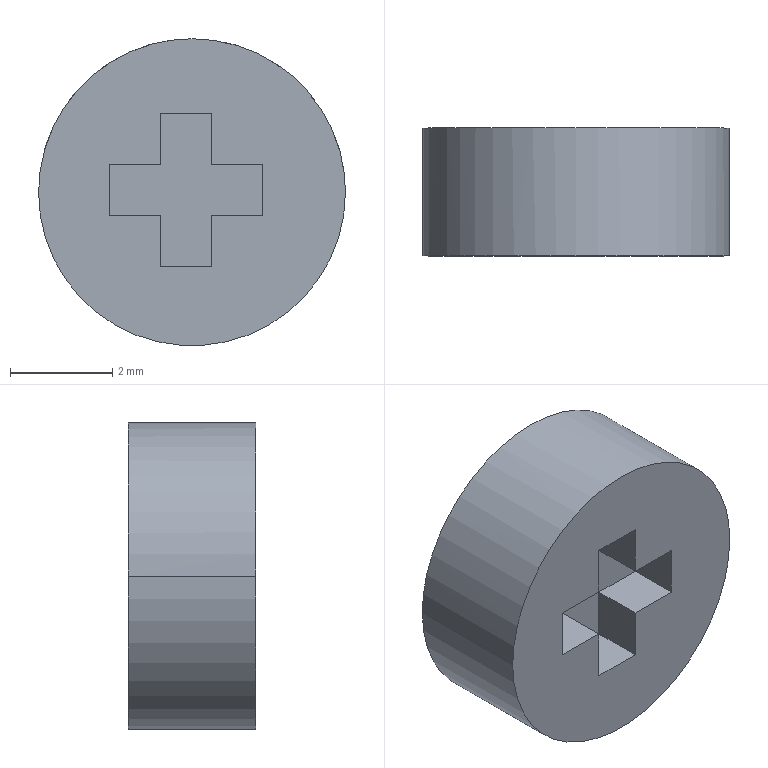Part | STEP file | Positioning_id1914_x_t | 1 solid | 17 faces | box 6 x 2.5 x 6 mm | volume 65.686 mm3 | plane 15 | cylinder 2 | commonest cylinder face diameters 6 x2
STEP:
#1=CARTESIAN_POINT('',(0.,0.,0.));
#2=DIRECTION('',(0.,0.,1.));
#3=DIRECTION('',(1.,0.,0.));
#4=AXIS2_PLACEMENT_3D('',#1,#2,#3);
#5=CARTESIAN_POINT('',(-766.532,-35.,479.288));
#6=VERTEX_POINT('',#5);
#7=CARTESIAN_POINT('',(-766.532,-35.,478.288));
#8=VERTEX_POINT('',#7);
#9=CARTESIAN_POINT('',(-766.532,-35.,479.288));
#10=DIRECTION('',(0.,0.,-1.));
#11=VECTOR('',#10,1.);
#12=LINE('',#9,#11);
#13=CARTESIAN_POINT('',(-766.532,-35.,478.288));
#14=DIRECTION('',(0.,1.,0.));
#15=DIRECTION('',(1.,0.,0.));
#16=AXIS2_PLACEMENT_3D('',#13,#14,#15);
#17=PLANE('',#16);
#18=CARTESIAN_POINT('',(0.,-1.));
#19=DIRECTION('',(0.,1.));
#20=VECTOR('',#19,1.);
#21=LINE('',#18,#20);
#22=(GEOMETRIC_REPRESENTATION_CONTEXT(2)PARAMETRIC_REPRESENTATION_CONTEXT()REPRESENTATION_CONTEXT('',''));
#23=DEFINITIONAL_REPRESENTATION('',(#21),#22);
#24=PCURVE('',#17,#23);
#25=CARTESIAN_POINT('',(-766.532,-35.,478.288));
#26=DIRECTION('',(-1.,0.,0.));
#27=DIRECTION('',(0.,0.,1.));
#28=AXIS2_PLACEMENT_3D('',#25,#26,#27);
#29=PLANE('',#28);
#30=CARTESIAN_POINT('',(1.,0.));
#31=DIRECTION('',(-1.,0.));
#32=VECTOR('',#31,1.);
#33=LINE('',#30,#32);
#34=(GEOMETRIC_REPRESENTATION_CONTEXT(2)PARAMETRIC_REPRESENTATION_CONTEXT()REPRESENTATION_CONTEXT('',''));
#35=DEFINITIONAL_REPRESENTATION('',(#33),#34);
#36=PCURVE('',#29,#35);
#37=SURFACE_CURVE('',#12,(#24,#36),.PCURVE_S1.);
#38=EDGE_CURVE('',#6,#8,#37,.T.);
#39=ORIENTED_EDGE('',*,*,#38,.F.);
#40=CARTESIAN_POINT('',(-767.532,-35.,479.288));
#41=VERTEX_POINT('',#40);
#42=CARTESIAN_POINT('',(-767.532,-35.,479.288));
#43=DIRECTION('',(1.,0.,0.));
#44=VECTOR('',#43,1.);
#45=LINE('',#42,#44);
#46=CARTESIAN_POINT('',(-1.,-1.));
#47=DIRECTION('',(1.,0.));
#48=VECTOR('',#47,1.);
#49=LINE('',#46,#48);
#50=(GEOMETRIC_REPRESENTATION_CONTEXT(2)PARAMETRIC_REPRESENTATION_CONTEXT()REPRESENTATION_CONTEXT('',''));
#51=DEFINITIONAL_REPRESENTATION('',(#49),#50);
#52=PCURVE('',#17,#51);
#53=CARTESIAN_POINT('',(-766.532,-35.,479.288));
#54=DIRECTION('',(0.,0.,-1.));
#55=DIRECTION('',(-1.,0.,0.));
#56=AXIS2_PLACEMENT_3D('',#53,#54,#55);
#57=PLANE('',#56);
#58=CARTESIAN_POINT('',(1.,0.));
#59=DIRECTION('',(-1.,0.));
#60=VECTOR('',#59,1.);
#61=LINE('',#58,#60);
#62=(GEOMETRIC_REPRESENTATION_CONTEXT(2)PARAMETRIC_REPRESENTATION_CONTEXT()REPRESENTATION_CONTEXT('',''));
#63=DEFINITIONAL_REPRESENTATION('',(#61),#62);
#64=PCURVE('',#57,#63);
#65=SURFACE_CURVE('',#45,(#52,#64),.PCURVE_S1.);
#66=EDGE_CURVE('',#41,#6,#65,.T.);
#67=ORIENTED_EDGE('',*,*,#66,.F.);
#68=CARTESIAN_POINT('',(-767.532,-35.,480.288));
#69=VERTEX_POINT('',#68);
#70=CARTESIAN_POINT('',(-767.532,-35.,480.288));
#71=DIRECTION('',(0.,0.,-1.));
#72=VECTOR('',#71,1.);
#73=LINE('',#70,#72);
#74=CARTESIAN_POINT('',(-1.,-2.));
#75=DIRECTION('',(0.,1.));
#76=VECTOR('',#75,1.);
#77=LINE('',#74,#76);
#78=(GEOMETRIC_REPRESENTATION_CONTEXT(2)PARAMETRIC_REPRESENTATION_CONTEXT()REPRESENTATION_CONTEXT('',''));
#79=DEFINITIONAL_REPRESENTATION('',(#77),#78);
#80=PCURVE('',#17,#79);
#81=CARTESIAN_POINT('',(-767.532,-35.,480.288));
#82=DIRECTION('',(-1.,0.,0.));
#83=DIRECTION('',(0.,0.,1.));
#84=AXIS2_PLACEMENT_3D('',#81,#82,#83);
#85=PLANE('',#84);
#86=CARTESIAN_POINT('',(0.,0.));
#87=DIRECTION('',(-1.,0.));
#88=VECTOR('',#87,1.);
#89=LINE('',#86,#88);
#90=(GEOMETRIC_REPRESENTATION_CONTEXT(2)PARAMETRIC_REPRESENTATION_CONTEXT()REPRESENTATION_CONTEXT('',''));
#91=DEFINITIONAL_REPRESENTATION('',(#89),#90);
#92=PCURVE('',#85,#91);
#93=SURFACE_CURVE('',#73,(#80,#92),.PCURVE_S1.);
#94=EDGE_CURVE('',#69,#41,#93,.T.);
#95=ORIENTED_EDGE('',*,*,#94,.F.);
#96=CARTESIAN_POINT('',(-768.532,-35.,480.288));
#97=VERTEX_POINT('',#96);
#98=CARTESIAN_POINT('',(-768.532,-35.,480.288));
#99=DIRECTION('',(1.,0.,0.));
#100=VECTOR('',#99,1.);
#101=LINE('',#98,#100);
#102=CARTESIAN_POINT('',(-2.,-2.));
#103=DIRECTION('',(1.,0.));
#104=VECTOR('',#103,1.);
#105=LINE('',#102,#104);
#106=(GEOMETRIC_REPRESENTATION_CONTEXT(2)PARAMETRIC_REPRESENTATION_CONTEXT()REPRESENTATION_CONTEXT('',''));
#107=DEFINITIONAL_REPRESENTATION('',(#105),#106);
#108=PCURVE('',#17,#107);
#109=CARTESIAN_POINT('',(-768.532,-35.,480.288));
#110=DIRECTION('',(0.,0.,-1.));
#111=DIRECTION('',(-1.,0.,0.));
#112=AXIS2_PLACEMENT_3D('',#109,#110,#111);
#113=PLANE('',#112);
#114=CARTESIAN_POINT('',(0.,0.));
#115=DIRECTION('',(-1.,0.));
#116=VECTOR('',#115,1.);
#117=LINE('',#114,#116);
#118=(GEOMETRIC_REPRESENTATION_CONTEXT(2)PARAMETRIC_REPRESENTATION_CONTEXT()REPRESENTATION_CONTEXT('',''));
#119=DEFINITIONAL_REPRESENTATION('',(#117),#118);
#120=PCURVE('',#113,#119);
#121=SURFACE_CURVE('',#101,(#108,#120),.PCURVE_S1.);
#122=EDGE_CURVE('',#97,#69,#121,.T.);
#123=ORIENTED_EDGE('',*,*,#122,.F.);
#124=CARTESIAN_POINT('',(-768.532,-35.,479.288));
#125=VERTEX_POINT('',#124);
#126=CARTESIAN_POINT('',(-768.532,-35.,479.288));
#127=DIRECTION('',(0.,0.,1.));
#128=VECTOR('',#127,1.);
#129=LINE('',#126,#128);
#130=CARTESIAN_POINT('',(-2.,-1.));
#131=DIRECTION('',(0.,-1.));
#132=VECTOR('',#131,1.);
#133=LINE('',#130,#132);
#134=(GEOMETRIC_REPRESENTATION_CONTEXT(2)PARAMETRIC_REPRESENTATION_CONTEXT()REPRESENTATION_CONTEXT('',''));
#135=DEFINITIONAL_REPRESENTATION('',(#133),#134);
#136=PCURVE('',#17,#135);
#137=CARTESIAN_POINT('',(-768.532,-35.,479.288));
#138=DIRECTION('',(1.,0.,0.));
#139=DIRECTION('',(0.,0.,-1.));
#140=AXIS2_PLACEMENT_3D('',#137,#138,#139);
#141=PLANE('',#140);
#142=CARTESIAN_POINT('',(0.,0.));
#143=DIRECTION('',(-1.,0.));
#144=VECTOR('',#143,1.);
#145=LINE('',#142,#144);
#146=(GEOMETRIC_REPRESENTATION_CONTEXT(2)PARAMETRIC_REPRESENTATION_CONTEXT()REPRESENTATION_CONTEXT('',''));
#147=DEFINITIONAL_REPRESENTATION('',(#145),#146);
#148=PCURVE('',#141,#147);
#149=SURFACE_CURVE('',#129,(#136,#148),.PCURVE_S1.);
#150=EDGE_CURVE('',#125,#97,#149,.T.);
#151=ORIENTED_EDGE('',*,*,#150,.F.);
#152=CARTESIAN_POINT('',(-769.532,-35.,479.288));
#153=VERTEX_POINT('',#152);
#154=CARTESIAN_POINT('',(-769.532,-35.,479.288));
#155=DIRECTION('',(1.,0.,0.));
#156=VECTOR('',#155,1.);
#157=LINE('',#154,#156);
#158=CARTESIAN_POINT('',(-3.,-1.));
#159=DIRECTION('',(1.,0.));
#160=VECTOR('',#159,1.);
#161=LINE('',#158,#160);
#162=(GEOMETRIC_REPRESENTATION_CONTEXT(2)PARAMETRIC_REPRESENTATION_CONTEXT()REPRESENTATION_CONTEXT('',''));
#163=DEFINITIONAL_REPRESENTATION('',(#161),#162);
#164=PCURVE('',#17,#163);
#165=CARTESIAN_POINT('',(-768.532,-35.,479.288));
#166=DIRECTION('',(0.,0.,-1.));
#167=DIRECTION('',(-1.,0.,0.));
#168=AXIS2_PLACEMENT_3D('',#165,#166,#167);
#169=PLANE('',#168);
#170=CARTESIAN_POINT('',(1.,0.));
#171=DIRECTION('',(-1.,0.));
#172=VECTOR('',#171,1.);
#173=LINE('',#170,#172);
#174=(GEOMETRIC_REPRESENTATION_CONTEXT(2)PARAMETRIC_REPRESENTATION_CONTEXT()REPRESENTATION_CONTEXT('',''));
#175=DEFINITIONAL_REPRESENTATION('',(#173),#174);
#176=PCURVE('',#169,#175);
#177=SURFACE_CURVE('',#157,(#164,#176),.PCURVE_S1.);
#178=EDGE_CURVE('',#153,#125,#177,.T.);
#179=ORIENTED_EDGE('',*,*,#178,.F.);
#180=CARTESIAN_POINT('',(-769.532,-35.,478.288));
#181=VERTEX_POINT('',#180);
#182=CARTESIAN_POINT('',(-769.532,-35.,478.288));
#183=DIRECTION('',(0.,0.,1.));
#184=VECTOR('',#183,1.);
#185=LINE('',#182,#184);
#186=CARTESIAN_POINT('',(-3.,0.));
#187=DIRECTION('',(0.,-1.));
#188=VECTOR('',#187,1.);
#189=LINE('',#186,#188);
#190=(GEOMETRIC_REPRESENTATION_CONTEXT(2)PARAMETRIC_REPRESENTATION_CONTEXT()REPRESENTATION_CONTEXT('',''));
#191=DEFINITIONAL_REPRESENTATION('',(#189),#190);
#192=PCURVE('',#17,#191);
#193=CARTESIAN_POINT('',(-769.532,-35.,479.288));
#194=DIRECTION('',(1.,0.,0.));
#195=DIRECTION('',(0.,0.,-1.));
#196=AXIS2_PLACEMENT_3D('',#193,#194,#195);
#197=PLANE('',#196);
#198=CARTESIAN_POINT('',(1.,0.));
#199=DIRECTION('',(-1.,0.));
#200=VECTOR('',#199,1.);
#201=LINE('',#198,#200);
#202=(GEOMETRIC_REPRESENTATION_CONTEXT(2)PARAMETRIC_REPRESENTATION_CONTEXT()REPRESENTATION_CONTEXT('',''));
#203=DEFINITIONAL_REPRESENTATION('',(#201),#202);
#204=PCURVE('',#197,#203);
#205=SURFACE_CURVE('',#185,(#192,#204),.PCURVE_S1.);
#206=EDGE_CURVE('',#181,#153,#205,.T.);
#207=ORIENTED_EDGE('',*,*,#206,.F.);
#208=CARTESIAN_POINT('',(-768.532,-35.,478.288));
#209=VERTEX_POINT('',#208);
#210=CARTESIAN_POINT('',(-768.532,-35.,478.288));
#211=DIRECTION('',(-1.,0.,0.));
#212=VECTOR('',#211,1.);
#213=LINE('',#210,#212);
#214=CARTESIAN_POINT('',(-2.,0.));
#215=DIRECTION('',(-1.,0.));
#216=VECTOR('',#215,1.);
#217=LINE('',#214,#216);
#218=(GEOMETRIC_REPRESENTATION_CONTEXT(2)PARAMETRIC_REPRESENTATION_CONTEXT()REPRESENTATION_CONTEXT('',''));
#219=DEFINITIONAL_REPRESENTATION('',(#217),#218);
#220=PCURVE('',#17,#219);
#221=CARTESIAN_POINT('',(-769.532,-35.,478.288));
#222=DIRECTION('',(0.,0.,1.));
#223=DIRECTION('',(1.,0.,0.));
#224=AXIS2_PLACEMENT_3D('',#221,#222,#223);
#225=PLANE('',#224);
#226=CARTESIAN_POINT('',(1.,0.));
#227=DIRECTION('',(-1.,0.));
#228=VECTOR('',#227,1.);
#229=LINE('',#226,#228);
#230=(GEOMETRIC_REPRESENTATION_CONTEXT(2)PARAMETRIC_REPRESENTATION_CONTEXT()REPRESENTATION_CONTEXT('',''));
#231=DEFINITIONAL_REPRESENTATION('',(#229),#230);
#232=PCURVE('',#225,#231);
#233=SURFACE_CURVE('',#213,(#220,#232),.PCURVE_S1.);
#234=EDGE_CURVE('',#209,#181,#233,.T.);
#235=ORIENTED_EDGE('',*,*,#234,.F.);
#236=CARTESIAN_POINT('',(-768.532,-35.,477.288));
#237=VERTEX_POINT('',#236);
#238=CARTESIAN_POINT('',(-768.532,-35.,477.288));
#239=DIRECTION('',(0.,0.,1.));
#240=VECTOR('',#239,1.);
#241=LINE('',#238,#240);
#242=CARTESIAN_POINT('',(-2.,1.));
#243=DIRECTION('',(0.,-1.));
#244=VECTOR('',#243,1.);
#245=LINE('',#242,#244);
#246=(GEOMETRIC_REPRESENTATION_CONTEXT(2)PARAMETRIC_REPRESENTATION_CONTEXT()REPRESENTATION_CONTEXT('',''));
#247=DEFINITIONAL_REPRESENTATION('',(#245),#246);
#248=PCURVE('',#17,#247);
#249=CARTESIAN_POINT('',(-768.532,-35.,477.288));
#250=DIRECTION('',(1.,0.,0.));
#251=DIRECTION('',(0.,0.,-1.));
#252=AXIS2_PLACEMENT_3D('',#249,#250,#251);
#253=PLANE('',#252);
#254=CARTESIAN_POINT('',(0.,0.));
#255=DIRECTION('',(-1.,0.));
#256=VECTOR('',#255,1.);
#257=LINE('',#254,#256);
#258=(GEOMETRIC_REPRESENTATION_CONTEXT(2)PARAMETRIC_REPRESENTATION_CONTEXT()REPRESENTATION_CONTEXT('',''));
#259=DEFINITIONAL_REPRESENTATION('',(#257),#258);
#260=PCURVE('',#253,#259);
#261=SURFACE_CURVE('',#241,(#248,#260),.PCURVE_S1.);
#262=EDGE_CURVE('',#237,#209,#261,.T.);
#263=ORIENTED_EDGE('',*,*,#262,.F.);
#264=CARTESIAN_POINT('',(-767.532,-35.,477.288));
#265=VERTEX_POINT('',#264);
#266=CARTESIAN_POINT('',(-767.532,-35.,477.288));
#267=DIRECTION('',(-1.,0.,0.));
#268=VECTOR('',#267,1.);
#269=LINE('',#266,#268);
#270=CARTESIAN_POINT('',(-1.,1.));
#271=DIRECTION('',(-1.,0.));
#272=VECTOR('',#271,1.);
#273=LINE('',#270,#272);
#274=(GEOMETRIC_REPRESENTATION_CONTEXT(2)PARAMETRIC_REPRESENTATION_CONTEXT()REPRESENTATION_CONTEXT('',''));
#275=DEFINITIONAL_REPRESENTATION('',(#273),#274);
#276=PCURVE('',#17,#275);
#277=CARTESIAN_POINT('',(-767.532,-35.,477.288));
#278=DIRECTION('',(0.,0.,1.));
#279=DIRECTION('',(1.,0.,0.));
#280=AXIS2_PLACEMENT_3D('',#277,#278,#279);
#281=PLANE('',#280);
#282=CARTESIAN_POINT('',(0.,0.));
#283=DIRECTION('',(-1.,0.));
#284=VECTOR('',#283,1.);
#285=LINE('',#282,#284);
#286=(GEOMETRIC_REPRESENTATION_CONTEXT(2)PARAMETRIC_REPRESENTATION_CONTEXT()REPRESENTATION_CONTEXT('',''));
#287=DEFINITIONAL_REPRESENTATION('',(#285),#286);
#288=PCURVE('',#281,#287);
#289=SURFACE_CURVE('',#269,(#276,#288),.PCURVE_S1.);
#290=EDGE_CURVE('',#265,#237,#289,.T.);
#291=ORIENTED_EDGE('',*,*,#290,.F.);
#292=CARTESIAN_POINT('',(-767.532,-35.,478.288));
#293=VERTEX_POINT('',#292);
#294=CARTESIAN_POINT('',(-767.532,-35.,478.288));
#295=DIRECTION('',(0.,0.,-1.));
#296=VECTOR('',#295,1.);
#297=LINE('',#294,#296);
#298=CARTESIAN_POINT('',(-1.,0.));
#299=DIRECTION('',(0.,1.));
#300=VECTOR('',#299,1.);
#301=LINE('',#298,#300);
#302=(GEOMETRIC_REPRESENTATION_CONTEXT(2)PARAMETRIC_REPRESENTATION_CONTEXT()REPRESENTATION_CONTEXT('',''));
#303=DEFINITIONAL_REPRESENTATION('',(#301),#302);
#304=PCURVE('',#17,#303);
#305=CARTESIAN_POINT('',(-767.532,-35.,478.288));
#306=DIRECTION('',(-1.,0.,0.));
#307=DIRECTION('',(0.,0.,1.));
#308=AXIS2_PLACEMENT_3D('',#305,#306,#307);
#309=PLANE('',#308);
#310=CARTESIAN_POINT('',(0.,0.));
#311=DIRECTION('',(-1.,0.));
#312=VECTOR('',#311,1.);
#313=LINE('',#310,#312);
#314=(GEOMETRIC_REPRESENTATION_CONTEXT(2)PARAMETRIC_REPRESENTATION_CONTEXT()REPRESENTATION_CONTEXT('',''));
#315=DEFINITIONAL_REPRESENTATION('',(#313),#314);
#316=PCURVE('',#309,#315);
#317=SURFACE_CURVE('',#297,(#304,#316),.PCURVE_S1.);
#318=EDGE_CURVE('',#293,#265,#317,.T.);
#319=ORIENTED_EDGE('',*,*,#318,.F.);
#320=CARTESIAN_POINT('',(-766.532,-35.,478.288));
#321=DIRECTION('',(-1.,0.,0.));
#322=VECTOR('',#321,1.);
#323=LINE('',#320,#322);
#324=CARTESIAN_POINT('',(0.,0.));
#325=DIRECTION('',(-1.,0.));
#326=VECTOR('',#325,1.);
#327=LINE('',#324,#326);
#328=(GEOMETRIC_REPRESENTATION_CONTEXT(2)PARAMETRIC_REPRESENTATION_CONTEXT()REPRESENTATION_CONTEXT('',''));
#329=DEFINITIONAL_REPRESENTATION('',(#327),#328);
#330=PCURVE('',#17,#329);
#331=CARTESIAN_POINT('',(-767.532,-35.,478.288));
#332=DIRECTION('',(0.,0.,1.));
#333=DIRECTION('',(1.,0.,0.));
#334=AXIS2_PLACEMENT_3D('',#331,#332,#333);
#335=PLANE('',#334);
#336=CARTESIAN_POINT('',(1.,0.));
#337=DIRECTION('',(-1.,0.));
#338=VECTOR('',#337,1.);
#339=LINE('',#336,#338);
#340=(GEOMETRIC_REPRESENTATION_CONTEXT(2)PARAMETRIC_REPRESENTATION_CONTEXT()REPRESENTATION_CONTEXT('',''));
#341=DEFINITIONAL_REPRESENTATION('',(#339),#340);
#342=PCURVE('',#335,#341);
#343=SURFACE_CURVE('',#323,(#330,#342),.PCURVE_S1.);
#344=EDGE_CURVE('',#8,#293,#343,.T.);
#345=ORIENTED_EDGE('',*,*,#344,.F.);
#346=EDGE_LOOP('',(#39,#67,#95,#123,#151,#179,#207,#235,#263,#291,#319,#345));
#347=FACE_BOUND('',#346,.T.);
#348=ADVANCED_FACE('',(#347),#17,.F.);
#349=ORIENTED_EDGE('',*,*,#66,.T.);
#350=CARTESIAN_POINT('',(-766.532,-36.,479.288));
#351=VERTEX_POINT('',#350);
#352=CARTESIAN_POINT('',(-766.532,-35.,479.288));
#353=DIRECTION('',(0.,-1.,0.));
#354=VECTOR('',#353,1.);
#355=LINE('',#352,#354);
#356=CARTESIAN_POINT('',(0.,0.));
#357=DIRECTION('',(0.,-1.));
#358=VECTOR('',#357,1.);
#359=LINE('',#356,#358);
#360=(GEOMETRIC_REPRESENTATION_CONTEXT(2)PARAMETRIC_REPRESENTATION_CONTEXT()REPRESENTATION_CONTEXT('',''));
#361=DEFINITIONAL_REPRESENTATION('',(#359),#360);
#362=PCURVE('',#57,#361);
#363=CARTESIAN_POINT('',(1.,0.));
#364=DIRECTION('',(0.,-1.));
#365=VECTOR('',#364,1.);
#366=LINE('',#363,#365);
#367=(GEOMETRIC_REPRESENTATION_CONTEXT(2)PARAMETRIC_REPRESENTATION_CONTEXT()REPRESENTATION_CONTEXT('',''));
#368=DEFINITIONAL_REPRESENTATION('',(#366),#367);
#369=PCURVE('',#29,#368);
#370=SURFACE_CURVE('',#355,(#362,#369),.PCURVE_S1.);
#371=EDGE_CURVE('',#6,#351,#370,.T.);
#372=ORIENTED_EDGE('',*,*,#371,.T.);
#373=CARTESIAN_POINT('',(-767.532,-36.,479.288));
#374=VERTEX_POINT('',#373);
#375=CARTESIAN_POINT('',(-767.532,-36.,479.288));
#376=DIRECTION('',(1.,0.,0.));
#377=VECTOR('',#376,1.);
#378=LINE('',#375,#377);
#379=CARTESIAN_POINT('',(1.,-1.));
#380=DIRECTION('',(-1.,0.));
#381=VECTOR('',#380,1.);
#382=LINE('',#379,#381);
#383=(GEOMETRIC_REPRESENTATION_CONTEXT(2)PARAMETRIC_REPRESENTATION_CONTEXT()REPRESENTATION_CONTEXT('',''));
#384=DEFINITIONAL_REPRESENTATION('',(#382),#383);
#385=PCURVE('',#57,#384);
#386=CARTESIAN_POINT('',(-767.916,-36.,478.74));
#387=DIRECTION('',(0.,1.,0.));
#388=DIRECTION('',(1.,0.,0.));
#389=AXIS2_PLACEMENT_3D('',#386,#387,#388);
#390=PLANE('',#389);
#391=CARTESIAN_POINT('',(0.3848,-0.5484));
#392=DIRECTION('',(1.,0.));
#393=VECTOR('',#392,1.);
#394=LINE('',#391,#393);
#395=(GEOMETRIC_REPRESENTATION_CONTEXT(2)PARAMETRIC_REPRESENTATION_CONTEXT()REPRESENTATION_CONTEXT('',''));
#396=DEFINITIONAL_REPRESENTATION('',(#394),#395);
#397=PCURVE('',#390,#396);
#398=SURFACE_CURVE('',#378,(#385,#397),.PCURVE_S1.);
#399=EDGE_CURVE('',#374,#351,#398,.T.);
#400=ORIENTED_EDGE('',*,*,#399,.F.);
#401=CARTESIAN_POINT('',(-767.532,-35.,479.288));
#402=DIRECTION('',(0.,-1.,0.));
#403=VECTOR('',#402,1.);
#404=LINE('',#401,#403);
#405=CARTESIAN_POINT('',(1.,0.));
#406=DIRECTION('',(0.,-1.));
#407=VECTOR('',#406,1.);
#408=LINE('',#405,#407);
#409=(GEOMETRIC_REPRESENTATION_CONTEXT(2)PARAMETRIC_REPRESENTATION_CONTEXT()REPRESENTATION_CONTEXT('',''));
#410=DEFINITIONAL_REPRESENTATION('',(#408),#409);
#411=PCURVE('',#57,#410);
#412=CARTESIAN_POINT('',(-1.,0.));
#413=DIRECTION('',(0.,-1.));
#414=VECTOR('',#413,1.);
#415=LINE('',#412,#414);
#416=(GEOMETRIC_REPRESENTATION_CONTEXT(2)PARAMETRIC_REPRESENTATION_CONTEXT()REPRESENTATION_CONTEXT('',''));
#417=DEFINITIONAL_REPRESENTATION('',(#415),#416);
#418=PCURVE('',#85,#417);
#419=SURFACE_CURVE('',#404,(#411,#418),.PCURVE_S1.);
#420=EDGE_CURVE('',#41,#374,#419,.T.);
#421=ORIENTED_EDGE('',*,*,#420,.F.);
#422=EDGE_LOOP('',(#349,#372,#400,#421));
#423=FACE_BOUND('',#422,.T.);
#424=ADVANCED_FACE('',(#423),#57,.T.);
#425=ORIENTED_EDGE('',*,*,#420,.T.);
#426=CARTESIAN_POINT('',(-767.532,-36.,480.288));
#427=VERTEX_POINT('',#426);
#428=CARTESIAN_POINT('',(-767.532,-36.,480.288));
#429=DIRECTION('',(0.,0.,-1.));
#430=VECTOR('',#429,1.);
#431=LINE('',#428,#430);
#432=CARTESIAN_POINT('',(0.,-1.));
#433=DIRECTION('',(-1.,0.));
#434=VECTOR('',#433,1.);
#435=LINE('',#432,#434);
#436=(GEOMETRIC_REPRESENTATION_CONTEXT(2)PARAMETRIC_REPRESENTATION_CONTEXT()REPRESENTATION_CONTEXT('',''));
#437=DEFINITIONAL_REPRESENTATION('',(#435),#436);
#438=PCURVE('',#85,#437);
#439=CARTESIAN_POINT('',(0.3848,-1.548));
#440=DIRECTION('',(0.,1.));
#441=VECTOR('',#440,1.);
#442=LINE('',#439,#441);
#443=(GEOMETRIC_REPRESENTATION_CONTEXT(2)PARAMETRIC_REPRESENTATION_CONTEXT()REPRESENTATION_CONTEXT('',''));
#444=DEFINITIONAL_REPRESENTATION('',(#442),#443);
#445=PCURVE('',#390,#444);
#446=SURFACE_CURVE('',#431,(#438,#445),.PCURVE_S1.);
#447=EDGE_CURVE('',#427,#374,#446,.T.);
#448=ORIENTED_EDGE('',*,*,#447,.F.);
#449=CARTESIAN_POINT('',(-767.532,-35.,480.288));
#450=DIRECTION('',(0.,-1.,0.));
#451=VECTOR('',#450,1.);
#452=LINE('',#449,#451);
#453=CARTESIAN_POINT('',(0.,0.));
#454=DIRECTION('',(0.,-1.));
#455=VECTOR('',#454,1.);
#456=LINE('',#453,#455);
#457=(GEOMETRIC_REPRESENTATION_CONTEXT(2)PARAMETRIC_REPRESENTATION_CONTEXT()REPRESENTATION_CONTEXT('',''));
#458=DEFINITIONAL_REPRESENTATION('',(#456),#457);
#459=PCURVE('',#85,#458);
#460=CARTESIAN_POINT('',(-1.,0.));
#461=DIRECTION('',(0.,-1.));
#462=VECTOR('',#461,1.);
#463=LINE('',#460,#462);
#464=(GEOMETRIC_REPRESENTATION_CONTEXT(2)PARAMETRIC_REPRESENTATION_CONTEXT()REPRESENTATION_CONTEXT('',''));
#465=DEFINITIONAL_REPRESENTATION('',(#463),#464);
#466=PCURVE('',#113,#465);
#467=SURFACE_CURVE('',#452,(#459,#466),.PCURVE_S1.);
#468=EDGE_CURVE('',#69,#427,#467,.T.);
#469=ORIENTED_EDGE('',*,*,#468,.F.);
#470=ORIENTED_EDGE('',*,*,#94,.T.);
#471=EDGE_LOOP('',(#425,#448,#469,#470));
#472=FACE_BOUND('',#471,.T.);
#473=ADVANCED_FACE('',(#472),#85,.T.);
#474=ORIENTED_EDGE('',*,*,#468,.T.);
#475=CARTESIAN_POINT('',(-768.532,-36.,480.288));
#476=VERTEX_POINT('',#475);
#477=CARTESIAN_POINT('',(-768.532,-36.,480.288));
#478=DIRECTION('',(1.,0.,0.));
#479=VECTOR('',#478,1.);
#480=LINE('',#477,#479);
#481=CARTESIAN_POINT('',(0.,-1.));
#482=DIRECTION('',(-1.,0.));
#483=VECTOR('',#482,1.);
#484=LINE('',#481,#483);
#485=(GEOMETRIC_REPRESENTATION_CONTEXT(2)PARAMETRIC_REPRESENTATION_CONTEXT()REPRESENTATION_CONTEXT('',''));
#486=DEFINITIONAL_REPRESENTATION('',(#484),#485);
#487=PCURVE('',#113,#486);
#488=CARTESIAN_POINT('',(-0.6152,-1.548));
#489=DIRECTION('',(1.,0.));
#490=VECTOR('',#489,1.);
#491=LINE('',#488,#490);
#492=(GEOMETRIC_REPRESENTATION_CONTEXT(2)PARAMETRIC_REPRESENTATION_CONTEXT()REPRESENTATION_CONTEXT('',''));
#493=DEFINITIONAL_REPRESENTATION('',(#491),#492);
#494=PCURVE('',#390,#493);
#495=SURFACE_CURVE('',#480,(#487,#494),.PCURVE_S1.);
#496=EDGE_CURVE('',#476,#427,#495,.T.);
#497=ORIENTED_EDGE('',*,*,#496,.F.);
#498=CARTESIAN_POINT('',(-768.532,-35.,480.288));
#499=DIRECTION('',(0.,-1.,0.));
#500=VECTOR('',#499,1.);
#501=LINE('',#498,#500);
#502=CARTESIAN_POINT('',(0.,0.));
#503=DIRECTION('',(0.,-1.));
#504=VECTOR('',#503,1.);
#505=LINE('',#502,#504);
#506=(GEOMETRIC_REPRESENTATION_CONTEXT(2)PARAMETRIC_REPRESENTATION_CONTEXT()REPRESENTATION_CONTEXT('',''));
#507=DEFINITIONAL_REPRESENTATION('',(#505),#506);
#508=PCURVE('',#113,#507);
#509=CARTESIAN_POINT('',(-1.,0.));
#510=DIRECTION('',(0.,-1.));
#511=VECTOR('',#510,1.);
#512=LINE('',#509,#511);
#513=(GEOMETRIC_REPRESENTATION_CONTEXT(2)PARAMETRIC_REPRESENTATION_CONTEXT()REPRESENTATION_CONTEXT('',''));
#514=DEFINITIONAL_REPRESENTATION('',(#512),#513);
#515=PCURVE('',#141,#514);
#516=SURFACE_CURVE('',#501,(#508,#515),.PCURVE_S1.);
#517=EDGE_CURVE('',#97,#476,#516,.T.);
#518=ORIENTED_EDGE('',*,*,#517,.F.);
#519=ORIENTED_EDGE('',*,*,#122,.T.);
#520=EDGE_LOOP('',(#474,#497,#518,#519));
#521=FACE_BOUND('',#520,.T.);
#522=ADVANCED_FACE('',(#521),#113,.T.);
#523=ORIENTED_EDGE('',*,*,#517,.T.);
#524=CARTESIAN_POINT('',(-768.532,-36.,479.288));
#525=VERTEX_POINT('',#524);
#526=CARTESIAN_POINT('',(-768.532,-36.,479.288));
#527=DIRECTION('',(0.,0.,1.));
#528=VECTOR('',#527,1.);
#529=LINE('',#526,#528);
#530=CARTESIAN_POINT('',(0.,-1.));
#531=DIRECTION('',(-1.,0.));
#532=VECTOR('',#531,1.);
#533=LINE('',#530,#532);
#534=(GEOMETRIC_REPRESENTATION_CONTEXT(2)PARAMETRIC_REPRESENTATION_CONTEXT()REPRESENTATION_CONTEXT('',''));
#535=DEFINITIONAL_REPRESENTATION('',(#533),#534);
#536=PCURVE('',#141,#535);
#537=CARTESIAN_POINT('',(-0.6152,-0.5484));
#538=DIRECTION('',(0.,-1.));
#539=VECTOR('',#538,1.);
#540=LINE('',#537,#539);
#541=(GEOMETRIC_REPRESENTATION_CONTEXT(2)PARAMETRIC_REPRESENTATION_CONTEXT()REPRESENTATION_CONTEXT('',''));
#542=DEFINITIONAL_REPRESENTATION('',(#540),#541);
#543=PCURVE('',#390,#542);
#544=SURFACE_CURVE('',#529,(#536,#543),.PCURVE_S1.);
#545=EDGE_CURVE('',#525,#476,#544,.T.);
#546=ORIENTED_EDGE('',*,*,#545,.F.);
#547=CARTESIAN_POINT('',(-768.532,-35.,479.288));
#548=DIRECTION('',(0.,-1.,0.));
#549=VECTOR('',#548,1.);
#550=LINE('',#547,#549);
#551=CARTESIAN_POINT('',(0.,0.));
#552=DIRECTION('',(0.,-1.));
#553=VECTOR('',#552,1.);
#554=LINE('',#551,#553);
#555=(GEOMETRIC_REPRESENTATION_CONTEXT(2)PARAMETRIC_REPRESENTATION_CONTEXT()REPRESENTATION_CONTEXT('',''));
#556=DEFINITIONAL_REPRESENTATION('',(#554),#555);
#557=PCURVE('',#141,#556);
#558=CARTESIAN_POINT('',(0.,0.));
#559=DIRECTION('',(0.,-1.));
#560=VECTOR('',#559,1.);
#561=LINE('',#558,#560);
#562=(GEOMETRIC_REPRESENTATION_CONTEXT(2)PARAMETRIC_REPRESENTATION_CONTEXT()REPRESENTATION_CONTEXT('',''));
#563=DEFINITIONAL_REPRESENTATION('',(#561),#562);
#564=PCURVE('',#169,#563);
#565=SURFACE_CURVE('',#550,(#557,#564),.PCURVE_S1.);
#566=EDGE_CURVE('',#125,#525,#565,.T.);
#567=ORIENTED_EDGE('',*,*,#566,.F.);
#568=ORIENTED_EDGE('',*,*,#150,.T.);
#569=EDGE_LOOP('',(#523,#546,#567,#568));
#570=FACE_BOUND('',#569,.T.);
#571=ADVANCED_FACE('',(#570),#141,.T.);
#572=ORIENTED_EDGE('',*,*,#566,.T.);
#573=CARTESIAN_POINT('',(-769.532,-36.,479.288));
#574=VERTEX_POINT('',#573);
#575=CARTESIAN_POINT('',(-769.532,-36.,479.288));
#576=DIRECTION('',(1.,0.,0.));
#577=VECTOR('',#576,1.);
#578=LINE('',#575,#577);
#579=CARTESIAN_POINT('',(1.,-1.));
#580=DIRECTION('',(-1.,0.));
#581=VECTOR('',#580,1.);
#582=LINE('',#579,#581);
#583=(GEOMETRIC_REPRESENTATION_CONTEXT(2)PARAMETRIC_REPRESENTATION_CONTEXT()REPRESENTATION_CONTEXT('',''));
#584=DEFINITIONAL_REPRESENTATION('',(#582),#583);
#585=PCURVE('',#169,#584);
#586=CARTESIAN_POINT('',(-1.615,-0.5484));
#587=DIRECTION('',(1.,0.));
#588=VECTOR('',#587,1.);
#589=LINE('',#586,#588);
#590=(GEOMETRIC_REPRESENTATION_CONTEXT(2)PARAMETRIC_REPRESENTATION_CONTEXT()REPRESENTATION_CONTEXT('',''));
#591=DEFINITIONAL_REPRESENTATION('',(#589),#590);
#592=PCURVE('',#390,#591);
#593=SURFACE_CURVE('',#578,(#585,#592),.PCURVE_S1.);
#594=EDGE_CURVE('',#574,#525,#593,.T.);
#595=ORIENTED_EDGE('',*,*,#594,.F.);
#596=CARTESIAN_POINT('',(-769.532,-35.,479.288));
#597=DIRECTION('',(0.,-1.,0.));
#598=VECTOR('',#597,1.);
#599=LINE('',#596,#598);
#600=CARTESIAN_POINT('',(1.,0.));
#601=DIRECTION('',(0.,-1.));
#602=VECTOR('',#601,1.);
#603=LINE('',#600,#602);
#604=(GEOMETRIC_REPRESENTATION_CONTEXT(2)PARAMETRIC_REPRESENTATION_CONTEXT()REPRESENTATION_CONTEXT('',''));
#605=DEFINITIONAL_REPRESENTATION('',(#603),#604);
#606=PCURVE('',#169,#605);
#607=CARTESIAN_POINT('',(0.,0.));
#608=DIRECTION('',(0.,-1.));
#609=VECTOR('',#608,1.);
#610=LINE('',#607,#609);
#611=(GEOMETRIC_REPRESENTATION_CONTEXT(2)PARAMETRIC_REPRESENTATION_CONTEXT()REPRESENTATION_CONTEXT('',''));
#612=DEFINITIONAL_REPRESENTATION('',(#610),#611);
#613=PCURVE('',#197,#612);
#614=SURFACE_CURVE('',#599,(#606,#613),.PCURVE_S1.);
#615=EDGE_CURVE('',#153,#574,#614,.T.);
#616=ORIENTED_EDGE('',*,*,#615,.F.);
#617=ORIENTED_EDGE('',*,*,#178,.T.);
#618=EDGE_LOOP('',(#572,#595,#616,#617));
#619=FACE_BOUND('',#618,.T.);
#620=ADVANCED_FACE('',(#619),#169,.T.);
#621=ORIENTED_EDGE('',*,*,#615,.T.);
#622=CARTESIAN_POINT('',(-769.532,-36.,478.288));
#623=VERTEX_POINT('',#622);
#624=CARTESIAN_POINT('',(-769.532,-36.,478.288));
#625=DIRECTION('',(0.,0.,1.));
#626=VECTOR('',#625,1.);
#627=LINE('',#624,#626);
#628=CARTESIAN_POINT('',(1.,-1.));
#629=DIRECTION('',(-1.,0.));
#630=VECTOR('',#629,1.);
#631=LINE('',#628,#630);
#632=(GEOMETRIC_REPRESENTATION_CONTEXT(2)PARAMETRIC_REPRESENTATION_CONTEXT()REPRESENTATION_CONTEXT('',''));
#633=DEFINITIONAL_REPRESENTATION('',(#631),#632);
#634=PCURVE('',#197,#633);
#635=CARTESIAN_POINT('',(-1.615,0.4516));
#636=DIRECTION('',(0.,-1.));
#637=VECTOR('',#636,1.);
#638=LINE('',#635,#637);
#639=(GEOMETRIC_REPRESENTATION_CONTEXT(2)PARAMETRIC_REPRESENTATION_CONTEXT()REPRESENTATION_CONTEXT('',''));
#640=DEFINITIONAL_REPRESENTATION('',(#638),#639);
#641=PCURVE('',#390,#640);
#642=SURFACE_CURVE('',#627,(#634,#641),.PCURVE_S1.);
#643=EDGE_CURVE('',#623,#574,#642,.T.);
#644=ORIENTED_EDGE('',*,*,#643,.F.);
#645=CARTESIAN_POINT('',(-769.532,-35.,478.288));
#646=DIRECTION('',(0.,-1.,0.));
#647=VECTOR('',#646,1.);
#648=LINE('',#645,#647);
#649=CARTESIAN_POINT('',(1.,0.));
#650=DIRECTION('',(0.,-1.));
#651=VECTOR('',#650,1.);
#652=LINE('',#649,#651);
#653=(GEOMETRIC_REPRESENTATION_CONTEXT(2)PARAMETRIC_REPRESENTATION_CONTEXT()REPRESENTATION_CONTEXT('',''));
#654=DEFINITIONAL_REPRESENTATION('',(#652),#653);
#655=PCURVE('',#197,#654);
#656=CARTESIAN_POINT('',(0.,0.));
#657=DIRECTION('',(0.,-1.));
#658=VECTOR('',#657,1.);
#659=LINE('',#656,#658);
#660=(GEOMETRIC_REPRESENTATION_CONTEXT(2)PARAMETRIC_REPRESENTATION_CONTEXT()REPRESENTATION_CONTEXT('',''));
#661=DEFINITIONAL_REPRESENTATION('',(#659),#660);
#662=PCURVE('',#225,#661);
#663=SURFACE_CURVE('',#648,(#655,#662),.PCURVE_S1.);
#664=EDGE_CURVE('',#181,#623,#663,.T.);
#665=ORIENTED_EDGE('',*,*,#664,.F.);
#666=ORIENTED_EDGE('',*,*,#206,.T.);
#667=EDGE_LOOP('',(#621,#644,#665,#666));
#668=FACE_BOUND('',#667,.T.);
#669=ADVANCED_FACE('',(#668),#197,.T.);
#670=ORIENTED_EDGE('',*,*,#664,.T.);
#671=CARTESIAN_POINT('',(-768.532,-36.,478.288));
#672=VERTEX_POINT('',#671);
#673=CARTESIAN_POINT('',(-768.532,-36.,478.288));
#674=DIRECTION('',(-1.,0.,0.));
#675=VECTOR('',#674,1.);
#676=LINE('',#673,#675);
#677=CARTESIAN_POINT('',(1.,-1.));
#678=DIRECTION('',(-1.,0.));
#679=VECTOR('',#678,1.);
#680=LINE('',#677,#679);
#681=(GEOMETRIC_REPRESENTATION_CONTEXT(2)PARAMETRIC_REPRESENTATION_CONTEXT()REPRESENTATION_CONTEXT('',''));
#682=DEFINITIONAL_REPRESENTATION('',(#680),#681);
#683=PCURVE('',#225,#682);
#684=CARTESIAN_POINT('',(-0.6152,0.4516));
#685=DIRECTION('',(-1.,0.));
#686=VECTOR('',#685,1.);
#687=LINE('',#684,#686);
#688=(GEOMETRIC_REPRESENTATION_CONTEXT(2)PARAMETRIC_REPRESENTATION_CONTEXT()REPRESENTATION_CONTEXT('',''));
#689=DEFINITIONAL_REPRESENTATION('',(#687),#688);
#690=PCURVE('',#390,#689);
#691=SURFACE_CURVE('',#676,(#683,#690),.PCURVE_S1.);
#692=EDGE_CURVE('',#672,#623,#691,.T.);
#693=ORIENTED_EDGE('',*,*,#692,.F.);
#694=CARTESIAN_POINT('',(-768.532,-35.,478.288));
#695=DIRECTION('',(0.,-1.,0.));
#696=VECTOR('',#695,1.);
#697=LINE('',#694,#696);
#698=CARTESIAN_POINT('',(1.,0.));
#699=DIRECTION('',(0.,-1.));
#700=VECTOR('',#699,1.);
#701=LINE('',#698,#700);
#702=(GEOMETRIC_REPRESENTATION_CONTEXT(2)PARAMETRIC_REPRESENTATION_CONTEXT()REPRESENTATION_CONTEXT('',''));
#703=DEFINITIONAL_REPRESENTATION('',(#701),#702);
#704=PCURVE('',#225,#703);
#705=CARTESIAN_POINT('',(-1.,0.));
#706=DIRECTION('',(0.,-1.));
#707=VECTOR('',#706,1.);
#708=LINE('',#705,#707);
#709=(GEOMETRIC_REPRESENTATION_CONTEXT(2)PARAMETRIC_REPRESENTATION_CONTEXT()REPRESENTATION_CONTEXT('',''));
#710=DEFINITIONAL_REPRESENTATION('',(#708),#709);
#711=PCURVE('',#253,#710);
#712=SURFACE_CURVE('',#697,(#704,#711),.PCURVE_S1.);
#713=EDGE_CURVE('',#209,#672,#712,.T.);
#714=ORIENTED_EDGE('',*,*,#713,.F.);
#715=ORIENTED_EDGE('',*,*,#234,.T.);
#716=EDGE_LOOP('',(#670,#693,#714,#715));
#717=FACE_BOUND('',#716,.T.);
#718=ADVANCED_FACE('',(#717),#225,.T.);
#719=ORIENTED_EDGE('',*,*,#713,.T.);
#720=CARTESIAN_POINT('',(-768.532,-36.,477.288));
#721=VERTEX_POINT('',#720);
#722=CARTESIAN_POINT('',(-768.532,-36.,477.288));
#723=DIRECTION('',(0.,0.,1.));
#724=VECTOR('',#723,1.);
#725=LINE('',#722,#724);
#726=CARTESIAN_POINT('',(0.,-1.));
#727=DIRECTION('',(-1.,0.));
#728=VECTOR('',#727,1.);
#729=LINE('',#726,#728);
#730=(GEOMETRIC_REPRESENTATION_CONTEXT(2)PARAMETRIC_REPRESENTATION_CONTEXT()REPRESENTATION_CONTEXT('',''));
#731=DEFINITIONAL_REPRESENTATION('',(#729),#730);
#732=PCURVE('',#253,#731);
#733=CARTESIAN_POINT('',(-0.6152,1.452));
#734=DIRECTION('',(0.,-1.));
#735=VECTOR('',#734,1.);
#736=LINE('',#733,#735);
#737=(GEOMETRIC_REPRESENTATION_CONTEXT(2)PARAMETRIC_REPRESENTATION_CONTEXT()REPRESENTATION_CONTEXT('',''));
#738=DEFINITIONAL_REPRESENTATION('',(#736),#737);
#739=PCURVE('',#390,#738);
#740=SURFACE_CURVE('',#725,(#732,#739),.PCURVE_S1.);
#741=EDGE_CURVE('',#721,#672,#740,.T.);
#742=ORIENTED_EDGE('',*,*,#741,.F.);
#743=CARTESIAN_POINT('',(-768.532,-35.,477.288));
#744=DIRECTION('',(0.,-1.,0.));
#745=VECTOR('',#744,1.);
#746=LINE('',#743,#745);
#747=CARTESIAN_POINT('',(0.,0.));
#748=DIRECTION('',(0.,-1.));
#749=VECTOR('',#748,1.);
#750=LINE('',#747,#749);
#751=(GEOMETRIC_REPRESENTATION_CONTEXT(2)PARAMETRIC_REPRESENTATION_CONTEXT()REPRESENTATION_CONTEXT('',''));
#752=DEFINITIONAL_REPRESENTATION('',(#750),#751);
#753=PCURVE('',#253,#752);
#754=CARTESIAN_POINT('',(-1.,0.));
#755=DIRECTION('',(0.,-1.));
#756=VECTOR('',#755,1.);
#757=LINE('',#754,#756);
#758=(GEOMETRIC_REPRESENTATION_CONTEXT(2)PARAMETRIC_REPRESENTATION_CONTEXT()REPRESENTATION_CONTEXT('',''));
#759=DEFINITIONAL_REPRESENTATION('',(#757),#758);
#760=PCURVE('',#281,#759);
#761=SURFACE_CURVE('',#746,(#753,#760),.PCURVE_S1.);
#762=EDGE_CURVE('',#237,#721,#761,.T.);
#763=ORIENTED_EDGE('',*,*,#762,.F.);
#764=ORIENTED_EDGE('',*,*,#262,.T.);
#765=EDGE_LOOP('',(#719,#742,#763,#764));
#766=FACE_BOUND('',#765,.T.);
#767=ADVANCED_FACE('',(#766),#253,.T.);
#768=ORIENTED_EDGE('',*,*,#762,.T.);
#769=CARTESIAN_POINT('',(-767.532,-36.,477.288));
#770=VERTEX_POINT('',#769);
#771=CARTESIAN_POINT('',(-767.532,-36.,477.288));
#772=DIRECTION('',(-1.,0.,0.));
#773=VECTOR('',#772,1.);
#774=LINE('',#771,#773);
#775=CARTESIAN_POINT('',(0.,-1.));
#776=DIRECTION('',(-1.,0.));
#777=VECTOR('',#776,1.);
#778=LINE('',#775,#777);
#779=(GEOMETRIC_REPRESENTATION_CONTEXT(2)PARAMETRIC_REPRESENTATION_CONTEXT()REPRESENTATION_CONTEXT('',''));
#780=DEFINITIONAL_REPRESENTATION('',(#778),#779);
#781=PCURVE('',#281,#780);
#782=CARTESIAN_POINT('',(0.3848,1.452));
#783=DIRECTION('',(-1.,0.));
#784=VECTOR('',#783,1.);
#785=LINE('',#782,#784);
#786=(GEOMETRIC_REPRESENTATION_CONTEXT(2)PARAMETRIC_REPRESENTATION_CONTEXT()REPRESENTATION_CONTEXT('',''));
#787=DEFINITIONAL_REPRESENTATION('',(#785),#786);
#788=PCURVE('',#390,#787);
#789=SURFACE_CURVE('',#774,(#781,#788),.PCURVE_S1.);
#790=EDGE_CURVE('',#770,#721,#789,.T.);
#791=ORIENTED_EDGE('',*,*,#790,.F.);
#792=CARTESIAN_POINT('',(-767.532,-35.,477.288));
#793=DIRECTION('',(0.,-1.,0.));
#794=VECTOR('',#793,1.);
#795=LINE('',#792,#794);
#796=CARTESIAN_POINT('',(0.,0.));
#797=DIRECTION('',(0.,-1.));
#798=VECTOR('',#797,1.);
#799=LINE('',#796,#798);
#800=(GEOMETRIC_REPRESENTATION_CONTEXT(2)PARAMETRIC_REPRESENTATION_CONTEXT()REPRESENTATION_CONTEXT('',''));
#801=DEFINITIONAL_REPRESENTATION('',(#799),#800);
#802=PCURVE('',#281,#801);
#803=CARTESIAN_POINT('',(-1.,0.));
#804=DIRECTION('',(0.,-1.));
#805=VECTOR('',#804,1.);
#806=LINE('',#803,#805);
#807=(GEOMETRIC_REPRESENTATION_CONTEXT(2)PARAMETRIC_REPRESENTATION_CONTEXT()REPRESENTATION_CONTEXT('',''));
#808=DEFINITIONAL_REPRESENTATION('',(#806),#807);
#809=PCURVE('',#309,#808);
#810=SURFACE_CURVE('',#795,(#802,#809),.PCURVE_S1.);
#811=EDGE_CURVE('',#265,#770,#810,.T.);
#812=ORIENTED_EDGE('',*,*,#811,.F.);
#813=ORIENTED_EDGE('',*,*,#290,.T.);
#814=EDGE_LOOP('',(#768,#791,#812,#813));
#815=FACE_BOUND('',#814,.T.);
#816=ADVANCED_FACE('',(#815),#281,.T.);
#817=ORIENTED_EDGE('',*,*,#811,.T.);
#818=CARTESIAN_POINT('',(-767.532,-36.,478.288));
#819=VERTEX_POINT('',#818);
#820=CARTESIAN_POINT('',(-767.532,-36.,478.288));
#821=DIRECTION('',(0.,0.,-1.));
#822=VECTOR('',#821,1.);
#823=LINE('',#820,#822);
#824=CARTESIAN_POINT('',(0.,-1.));
#825=DIRECTION('',(-1.,0.));
#826=VECTOR('',#825,1.);
#827=LINE('',#824,#826);
#828=(GEOMETRIC_REPRESENTATION_CONTEXT(2)PARAMETRIC_REPRESENTATION_CONTEXT()REPRESENTATION_CONTEXT('',''));
#829=DEFINITIONAL_REPRESENTATION('',(#827),#828);
#830=PCURVE('',#309,#829);
#831=CARTESIAN_POINT('',(0.3848,0.4516));
#832=DIRECTION('',(0.,1.));
#833=VECTOR('',#832,1.);
#834=LINE('',#831,#833);
#835=(GEOMETRIC_REPRESENTATION_CONTEXT(2)PARAMETRIC_REPRESENTATION_CONTEXT()REPRESENTATION_CONTEXT('',''));
#836=DEFINITIONAL_REPRESENTATION('',(#834),#835);
#837=PCURVE('',#390,#836);
#838=SURFACE_CURVE('',#823,(#830,#837),.PCURVE_S1.);
#839=EDGE_CURVE('',#819,#770,#838,.T.);
#840=ORIENTED_EDGE('',*,*,#839,.F.);
#841=CARTESIAN_POINT('',(-767.532,-35.,478.288));
#842=DIRECTION('',(0.,-1.,0.));
#843=VECTOR('',#842,1.);
#844=LINE('',#841,#843);
#845=CARTESIAN_POINT('',(0.,0.));
#846=DIRECTION('',(0.,-1.));
#847=VECTOR('',#846,1.);
#848=LINE('',#845,#847);
#849=(GEOMETRIC_REPRESENTATION_CONTEXT(2)PARAMETRIC_REPRESENTATION_CONTEXT()REPRESENTATION_CONTEXT('',''));
#850=DEFINITIONAL_REPRESENTATION('',(#848),#849);
#851=PCURVE('',#309,#850);
#852=CARTESIAN_POINT('',(0.,0.));
#853=DIRECTION('',(0.,-1.));
#854=VECTOR('',#853,1.);
#855=LINE('',#852,#854);
#856=(GEOMETRIC_REPRESENTATION_CONTEXT(2)PARAMETRIC_REPRESENTATION_CONTEXT()REPRESENTATION_CONTEXT('',''));
#857=DEFINITIONAL_REPRESENTATION('',(#855),#856);
#858=PCURVE('',#335,#857);
#859=SURFACE_CURVE('',#844,(#851,#858),.PCURVE_S1.);
#860=EDGE_CURVE('',#293,#819,#859,.T.);
#861=ORIENTED_EDGE('',*,*,#860,.F.);
#862=ORIENTED_EDGE('',*,*,#318,.T.);
#863=EDGE_LOOP('',(#817,#840,#861,#862));
#864=FACE_BOUND('',#863,.T.);
#865=ADVANCED_FACE('',(#864),#309,.T.);
#866=ORIENTED_EDGE('',*,*,#860,.T.);
#867=CARTESIAN_POINT('',(-766.532,-36.,478.288));
#868=VERTEX_POINT('',#867);
#869=CARTESIAN_POINT('',(-766.532,-36.,478.288));
#870=DIRECTION('',(-1.,0.,0.));
#871=VECTOR('',#870,1.);
#872=LINE('',#869,#871);
#873=CARTESIAN_POINT('',(1.,-1.));
#874=DIRECTION('',(-1.,0.));
#875=VECTOR('',#874,1.);
#876=LINE('',#873,#875);
#877=(GEOMETRIC_REPRESENTATION_CONTEXT(2)PARAMETRIC_REPRESENTATION_CONTEXT()REPRESENTATION_CONTEXT('',''));
#878=DEFINITIONAL_REPRESENTATION('',(#876),#877);
#879=PCURVE('',#335,#878);
#880=CARTESIAN_POINT('',(1.385,0.4516));
#881=DIRECTION('',(-1.,0.));
#882=VECTOR('',#881,1.);
#883=LINE('',#880,#882);
#884=(GEOMETRIC_REPRESENTATION_CONTEXT(2)PARAMETRIC_REPRESENTATION_CONTEXT()REPRESENTATION_CONTEXT('',''));
#885=DEFINITIONAL_REPRESENTATION('',(#883),#884);
#886=PCURVE('',#390,#885);
#887=SURFACE_CURVE('',#872,(#879,#886),.PCURVE_S1.);
#888=EDGE_CURVE('',#868,#819,#887,.T.);
#889=ORIENTED_EDGE('',*,*,#888,.F.);
#890=CARTESIAN_POINT('',(-766.532,-35.,478.288));
#891=DIRECTION('',(0.,-1.,0.));
#892=VECTOR('',#891,1.);
#893=LINE('',#890,#892);
#894=CARTESIAN_POINT('',(1.,0.));
#895=DIRECTION('',(0.,-1.));
#896=VECTOR('',#895,1.);
#897=LINE('',#894,#896);
#898=(GEOMETRIC_REPRESENTATION_CONTEXT(2)PARAMETRIC_REPRESENTATION_CONTEXT()REPRESENTATION_CONTEXT('',''));
#899=DEFINITIONAL_REPRESENTATION('',(#897),#898);
#900=PCURVE('',#335,#899);
#901=CARTESIAN_POINT('',(0.,0.));
#902=DIRECTION('',(0.,-1.));
#903=VECTOR('',#902,1.);
#904=LINE('',#901,#903);
#905=(GEOMETRIC_REPRESENTATION_CONTEXT(2)PARAMETRIC_REPRESENTATION_CONTEXT()REPRESENTATION_CONTEXT('',''));
#906=DEFINITIONAL_REPRESENTATION('',(#904),#905);
#907=PCURVE('',#29,#906);
#908=SURFACE_CURVE('',#893,(#900,#907),.PCURVE_S1.);
#909=EDGE_CURVE('',#8,#868,#908,.T.);
#910=ORIENTED_EDGE('',*,*,#909,.F.);
#911=ORIENTED_EDGE('',*,*,#344,.T.);
#912=EDGE_LOOP('',(#866,#889,#910,#911));
#913=FACE_BOUND('',#912,.T.);
#914=ADVANCED_FACE('',(#913),#335,.T.);
#915=ORIENTED_EDGE('',*,*,#909,.T.);
#916=CARTESIAN_POINT('',(-766.532,-36.,479.288));
#917=DIRECTION('',(0.,0.,-1.));
#918=VECTOR('',#917,1.);
#919=LINE('',#916,#918);
#920=CARTESIAN_POINT('',(1.,-1.));
#921=DIRECTION('',(-1.,0.));
#922=VECTOR('',#921,1.);
#923=LINE('',#920,#922);
#924=(GEOMETRIC_REPRESENTATION_CONTEXT(2)PARAMETRIC_REPRESENTATION_CONTEXT()REPRESENTATION_CONTEXT('',''));
#925=DEFINITIONAL_REPRESENTATION('',(#923),#924);
#926=PCURVE('',#29,#925);
#927=CARTESIAN_POINT('',(1.385,-0.5484));
#928=DIRECTION('',(0.,1.));
#929=VECTOR('',#928,1.);
#930=LINE('',#927,#929);
#931=(GEOMETRIC_REPRESENTATION_CONTEXT(2)PARAMETRIC_REPRESENTATION_CONTEXT()REPRESENTATION_CONTEXT('',''));
#932=DEFINITIONAL_REPRESENTATION('',(#930),#931);
#933=PCURVE('',#390,#932);
#934=SURFACE_CURVE('',#919,(#926,#933),.PCURVE_S1.);
#935=EDGE_CURVE('',#351,#868,#934,.T.);
#936=ORIENTED_EDGE('',*,*,#935,.F.);
#937=ORIENTED_EDGE('',*,*,#371,.F.);
#938=ORIENTED_EDGE('',*,*,#38,.T.);
#939=EDGE_LOOP('',(#915,#936,#937,#938));
#940=FACE_BOUND('',#939,.T.);
#941=ADVANCED_FACE('',(#940),#29,.T.);
#942=CARTESIAN_POINT('',(-770.916,-33.5,478.74));
#943=VERTEX_POINT('',#942);
#944=CARTESIAN_POINT('',(-767.916,-33.5,481.74));
#945=VERTEX_POINT('',#944);
#946=CARTESIAN_POINT('',(-767.916,-33.5,478.74));
#947=DIRECTION('',(0.,1.,0.));
#948=DIRECTION('',(-1.,0.,0.));
#949=AXIS2_PLACEMENT_3D('',#946,#947,#948);
#950=CIRCLE('',#949,3.);
#951=CARTESIAN_POINT('',(-767.916,-33.5,478.74));
#952=DIRECTION('',(0.,1.,0.));
#953=DIRECTION('',(1.,0.,0.));
#954=AXIS2_PLACEMENT_3D('',#951,#952,#953);
#955=PLANE('',#954);
#956=CARTESIAN_POINT('',(0.,0.));
#957=DIRECTION('',(-1.,0.));
#958=AXIS2_PLACEMENT_2D('',#956,#957);
#959=CIRCLE('',#958,3.);
#960=(GEOMETRIC_REPRESENTATION_CONTEXT(2)PARAMETRIC_REPRESENTATION_CONTEXT()REPRESENTATION_CONTEXT('',''));
#961=DEFINITIONAL_REPRESENTATION('',(#959),#960);
#962=PCURVE('',#955,#961);
#963=CARTESIAN_POINT('',(-767.916,-36.,478.74));
#964=DIRECTION('',(0.,-1.,0.));
#965=DIRECTION('',(1.,0.,0.));
#966=AXIS2_PLACEMENT_3D('',#963,#964,#965);
#967=CYLINDRICAL_SURFACE('',#966,3.);
#968=CARTESIAN_POINT('',(3.142,-2.5));
#969=DIRECTION('',(-1.,0.));
#970=VECTOR('',#969,1.);
#971=LINE('',#968,#970);
#972=(GEOMETRIC_REPRESENTATION_CONTEXT(2)PARAMETRIC_REPRESENTATION_CONTEXT()REPRESENTATION_CONTEXT('',''));
#973=DEFINITIONAL_REPRESENTATION('',(#971),#972);
#974=PCURVE('',#967,#973);
#975=SURFACE_CURVE('',#950,(#962,#974),.PCURVE_S1.);
#976=EDGE_CURVE('',#943,#945,#975,.T.);
#977=ORIENTED_EDGE('',*,*,#976,.T.);
#978=CARTESIAN_POINT('',(-764.916,-33.5,478.74));
#979=VERTEX_POINT('',#978);
#980=CARTESIAN_POINT('',(-767.916,-33.5,478.74));
#981=DIRECTION('',(0.,1.,0.));
#982=DIRECTION('',(0.,0.,1.));
#983=AXIS2_PLACEMENT_3D('',#980,#981,#982);
#984=CIRCLE('',#983,3.);
#985=CARTESIAN_POINT('',(0.,0.));
#986=DIRECTION('',(0.,-1.));
#987=AXIS2_PLACEMENT_2D('',#985,#986);
#988=CIRCLE('',#987,3.);
#989=(GEOMETRIC_REPRESENTATION_CONTEXT(2)PARAMETRIC_REPRESENTATION_CONTEXT()REPRESENTATION_CONTEXT('',''));
#990=DEFINITIONAL_REPRESENTATION('',(#988),#989);
#991=PCURVE('',#955,#990);
#992=CARTESIAN_POINT('',(1.571,-2.5));
#993=DIRECTION('',(-1.,0.));
#994=VECTOR('',#993,1.);
#995=LINE('',#992,#994);
#996=(GEOMETRIC_REPRESENTATION_CONTEXT(2)PARAMETRIC_REPRESENTATION_CONTEXT()REPRESENTATION_CONTEXT('',''));
#997=DEFINITIONAL_REPRESENTATION('',(#995),#996);
#998=PCURVE('',#967,#997);
#999=SURFACE_CURVE('',#984,(#991,#998),.PCURVE_S1.);
#1000=EDGE_CURVE('',#945,#979,#999,.T.);
#1001=ORIENTED_EDGE('',*,*,#1000,.T.);
#1002=CARTESIAN_POINT('',(-767.916,-33.5,478.74));
#1003=DIRECTION('',(0.,1.,0.));
#1004=DIRECTION('',(1.,0.,0.));
#1005=AXIS2_PLACEMENT_3D('',#1002,#1003,#1004);
#1006=CIRCLE('',#1005,3.);
#1007=CARTESIAN_POINT('',(0.,0.));
#1008=DIRECTION('',(1.,0.));
#1009=AXIS2_PLACEMENT_2D('',#1007,#1008);
#1010=CIRCLE('',#1009,3.);
#1011=(GEOMETRIC_REPRESENTATION_CONTEXT(2)PARAMETRIC_REPRESENTATION_CONTEXT()REPRESENTATION_CONTEXT('',''));
#1012=DEFINITIONAL_REPRESENTATION('',(#1010),#1011);
#1013=PCURVE('',#955,#1012);
#1014=CARTESIAN_POINT('',(-767.916,-36.,478.74));
#1015=DIRECTION('',(0.,-1.,0.));
#1016=DIRECTION('',(1.,0.,0.));
#1017=AXIS2_PLACEMENT_3D('',#1014,#1015,#1016);
#1018=CYLINDRICAL_SURFACE('',#1017,3.);
#1019=CARTESIAN_POINT('',(6.283,-2.5));
#1020=DIRECTION('',(-1.,0.));
#1021=VECTOR('',#1020,1.);
#1022=LINE('',#1019,#1021);
#1023=(GEOMETRIC_REPRESENTATION_CONTEXT(2)PARAMETRIC_REPRESENTATION_CONTEXT()REPRESENTATION_CONTEXT('',''));
#1024=DEFINITIONAL_REPRESENTATION('',(#1022),#1023);
#1025=PCURVE('',#1018,#1024);
#1026=SURFACE_CURVE('',#1006,(#1013,#1025),.PCURVE_S1.);
#1027=EDGE_CURVE('',#979,#943,#1026,.T.);
#1028=ORIENTED_EDGE('',*,*,#1027,.T.);
#1029=EDGE_LOOP('',(#977,#1001,#1028));
#1030=FACE_BOUND('',#1029,.T.);
#1031=ADVANCED_FACE('',(#1030),#955,.T.);
#1032=CARTESIAN_POINT('',(-764.916,-36.,478.74));
#1033=VERTEX_POINT('',#1032);
#1034=CARTESIAN_POINT('',(-764.916,-36.,478.74));
#1035=DIRECTION('',(0.,1.,0.));
#1036=VECTOR('',#1035,1.);
#1037=LINE('',#1034,#1036);
#1038=CARTESIAN_POINT('',(6.283,0.));
#1039=DIRECTION('',(0.,-1.));
#1040=VECTOR('',#1039,1.);
#1041=LINE('',#1038,#1040);
#1042=(GEOMETRIC_REPRESENTATION_CONTEXT(2)PARAMETRIC_REPRESENTATION_CONTEXT()REPRESENTATION_CONTEXT('',''));
#1043=DEFINITIONAL_REPRESENTATION('',(#1041),#1042);
#1044=PCURVE('',#1018,#1043);
#1045=CARTESIAN_POINT('',(0.,0.));
#1046=DIRECTION('',(0.,-1.));
#1047=VECTOR('',#1046,1.);
#1048=LINE('',#1045,#1047);
#1049=(GEOMETRIC_REPRESENTATION_CONTEXT(2)PARAMETRIC_REPRESENTATION_CONTEXT()REPRESENTATION_CONTEXT('',''));
#1050=DEFINITIONAL_REPRESENTATION('',(#1048),#1049);
#1051=PCURVE('',#967,#1050);
#1052=SURFACE_CURVE('',#1037,(#1044,#1051),.PCURVE_S1.);
#1053=EDGE_CURVE('',#1033,#979,#1052,.T.);
#1054=ORIENTED_EDGE('',*,*,#1053,.F.);
#1055=CARTESIAN_POINT('',(-770.916,-36.,478.74));
#1056=VERTEX_POINT('',#1055);
#1057=CARTESIAN_POINT('',(-767.916,-36.,478.74));
#1058=DIRECTION('',(0.,1.,0.));
#1059=DIRECTION('',(1.,0.,0.));
#1060=AXIS2_PLACEMENT_3D('',#1057,#1058,#1059);
#1061=CIRCLE('',#1060,3.);
#1062=CARTESIAN_POINT('',(6.283,0.));
#1063=DIRECTION('',(-1.,0.));
#1064=VECTOR('',#1063,1.);
#1065=LINE('',#1062,#1064);
#1066=(GEOMETRIC_REPRESENTATION_CONTEXT(2)PARAMETRIC_REPRESENTATION_CONTEXT()REPRESENTATION_CONTEXT('',''));
#1067=DEFINITIONAL_REPRESENTATION('',(#1065),#1066);
#1068=PCURVE('',#1018,#1067);
#1069=CARTESIAN_POINT('',(0.,0.));
#1070=DIRECTION('',(1.,0.));
#1071=AXIS2_PLACEMENT_2D('',#1069,#1070);
#1072=CIRCLE('',#1071,3.);
#1073=(GEOMETRIC_REPRESENTATION_CONTEXT(2)PARAMETRIC_REPRESENTATION_CONTEXT()REPRESENTATION_CONTEXT('',''));
#1074=DEFINITIONAL_REPRESENTATION('',(#1072),#1073);
#1075=PCURVE('',#390,#1074);
#1076=SURFACE_CURVE('',#1061,(#1068,#1075),.PCURVE_S1.);
#1077=EDGE_CURVE('',#1033,#1056,#1076,.T.);
#1078=ORIENTED_EDGE('',*,*,#1077,.T.);
#1079=CARTESIAN_POINT('',(-770.916,-36.,478.74));
#1080=DIRECTION('',(0.,-1.,0.));
#1081=VECTOR('',#1080,1.);
#1082=LINE('',#1079,#1081);
#1083=CARTESIAN_POINT('',(3.142,0.));
#1084=DIRECTION('',(0.,1.));
#1085=VECTOR('',#1084,1.);
#1086=LINE('',#1083,#1085);
#1087=(GEOMETRIC_REPRESENTATION_CONTEXT(2)PARAMETRIC_REPRESENTATION_CONTEXT()REPRESENTATION_CONTEXT('',''));
#1088=DEFINITIONAL_REPRESENTATION('',(#1086),#1087);
#1089=PCURVE('',#1018,#1088);
#1090=CARTESIAN_POINT('',(3.142,0.));
#1091=DIRECTION('',(0.,1.));
#1092=VECTOR('',#1091,1.);
#1093=LINE('',#1090,#1092);
#1094=(GEOMETRIC_REPRESENTATION_CONTEXT(2)PARAMETRIC_REPRESENTATION_CONTEXT()REPRESENTATION_CONTEXT('',''));
#1095=DEFINITIONAL_REPRESENTATION('',(#1093),#1094);
#1096=PCURVE('',#967,#1095);
#1097=SURFACE_CURVE('',#1082,(#1089,#1096),.PCURVE_S1.);
#1098=EDGE_CURVE('',#943,#1056,#1097,.T.);
#1099=ORIENTED_EDGE('',*,*,#1098,.F.);
#1100=ORIENTED_EDGE('',*,*,#1027,.F.);
#1101=EDGE_LOOP('',(#1054,#1078,#1099,#1100));
#1102=FACE_BOUND('',#1101,.T.);
#1103=ADVANCED_FACE('',(#1102),#1018,.T.);
#1104=ORIENTED_EDGE('',*,*,#935,.T.);
#1105=ORIENTED_EDGE('',*,*,#888,.T.);
#1106=ORIENTED_EDGE('',*,*,#839,.T.);
#1107=ORIENTED_EDGE('',*,*,#790,.T.);
#1108=ORIENTED_EDGE('',*,*,#741,.T.);
#1109=ORIENTED_EDGE('',*,*,#692,.T.);
#1110=ORIENTED_EDGE('',*,*,#643,.T.);
#1111=ORIENTED_EDGE('',*,*,#594,.T.);
#1112=ORIENTED_EDGE('',*,*,#545,.T.);
#1113=ORIENTED_EDGE('',*,*,#496,.T.);
#1114=ORIENTED_EDGE('',*,*,#447,.T.);
#1115=ORIENTED_EDGE('',*,*,#399,.T.);
#1116=EDGE_LOOP('',(#1104,#1105,#1106,#1107,#1108,#1109,#1110,#1111,#1112,#1113,#1114,#1115));
#1117=FACE_BOUND('',#1116,.T.);
#1118=CARTESIAN_POINT('',(-767.916,-36.,481.74));
#1119=VERTEX_POINT('',#1118);
#1120=CARTESIAN_POINT('',(-770.916,-36.,478.74));
#1121=CARTESIAN_POINT('',(-770.916,-36.,481.74));
#1122=CARTESIAN_POINT('',(-767.916,-36.,481.74));
#1123=(BOUNDED_CURVE()B_SPLINE_CURVE(2,(#1120,#1121,#1122),.UNSPECIFIED.,.F.,.F.)B_SPLINE_CURVE_WITH_KNOTS((3,3),(0.,1.),.PIECEWISE_BEZIER_KNOTS.)CURVE()GEOMETRIC_REPRESENTATION_ITEM()RATIONAL_B_SPLINE_CURVE((1.,0.7071,1.))REPRESENTATION_ITEM(''));
#1124=CARTESIAN_POINT('',(-3.,0.));
#1125=CARTESIAN_POINT('',(-3.,-3.));
#1126=CARTESIAN_POINT('',(0.,-3.));
#1127=(BOUNDED_CURVE()B_SPLINE_CURVE(2,(#1124,#1125,#1126),.UNSPECIFIED.,.F.,.F.)B_SPLINE_CURVE_WITH_KNOTS((3,3),(0.,1.),.PIECEWISE_BEZIER_KNOTS.)CURVE()GEOMETRIC_REPRESENTATION_ITEM()RATIONAL_B_SPLINE_CURVE((1.,0.7071,1.))REPRESENTATION_ITEM(''));
#1128=(GEOMETRIC_REPRESENTATION_CONTEXT(2)PARAMETRIC_REPRESENTATION_CONTEXT()REPRESENTATION_CONTEXT('',''));
#1129=DEFINITIONAL_REPRESENTATION('',(#1127),#1128);
#1130=PCURVE('',#390,#1129);
#1131=CARTESIAN_POINT('',(3.142,0.));
#1132=CARTESIAN_POINT('',(3.12,0.));
#1133=CARTESIAN_POINT('',(3.077,0.));
#1134=CARTESIAN_POINT('',(3.01,0.));
#1135=CARTESIAN_POINT('',(2.942,0.));
#1136=CARTESIAN_POINT('',(2.872,0.));
#1137=CARTESIAN_POINT('',(2.801,0.));
#1138=CARTESIAN_POINT('',(2.729,0.));
#1139=CARTESIAN_POINT('',(2.655,0.));
#1140=CARTESIAN_POINT('',(2.581,0.));
#1141=CARTESIAN_POINT('',(2.507,0.));
#1142=CARTESIAN_POINT('',(2.432,0.));
#1143=CARTESIAN_POINT('',(2.356,0.));
#1144=CARTESIAN_POINT('',(2.281,0.));
#1145=CARTESIAN_POINT('',(2.206,0.));
#1146=CARTESIAN_POINT('',(2.131,0.));
#1147=CARTESIAN_POINT('',(2.057,0.));
#1148=CARTESIAN_POINT('',(1.984,0.));
#1149=CARTESIAN_POINT('',(1.912,0.));
#1150=CARTESIAN_POINT('',(1.841,0.));
#1151=CARTESIAN_POINT('',(1.771,0.));
#1152=CARTESIAN_POINT('',(1.702,0.));
#1153=CARTESIAN_POINT('',(1.636,0.));
#1154=CARTESIAN_POINT('',(1.592,0.));
#1155=CARTESIAN_POINT('',(1.571,0.));
#1156=B_SPLINE_CURVE_WITH_KNOTS('',3,(#1131,#1132,#1133,#1134,#1135,#1136,#1137,#1138,#1139,#1140,#1141,#1142,#1143,#1144,#1145,#1146,#1147,#1148,#1149,#1150,#1151,#1152,#1153,#1154,#1155),.UNSPECIFIED.,.F.,.F.,(4,1,1,1,1,1,1,1,1,1,1,1,1,1,1,1,1,1,1,1,1,1,4),(0.,0.04545,0.09091,0.1364,0.1818,0.2273,0.2727,0.3182,0.3636,0.4091,0.4545,0.5,0.5455,0.5909,0.6364,0.6818,0.7273,0.7727,0.8182,0.8636,0.9091,0.9545,1.),.QUASI_UNIFORM_KNOTS.);
#1157=(GEOMETRIC_REPRESENTATION_CONTEXT(2)PARAMETRIC_REPRESENTATION_CONTEXT()REPRESENTATION_CONTEXT('',''));
#1158=DEFINITIONAL_REPRESENTATION('',(#1156),#1157);
#1159=PCURVE('',#967,#1158);
#1160=SURFACE_CURVE('',#1123,(#1130,#1159),.PCURVE_S1.);
#1161=EDGE_CURVE('',#1056,#1119,#1160,.T.);
#1162=ORIENTED_EDGE('',*,*,#1161,.F.);
#1163=ORIENTED_EDGE('',*,*,#1077,.F.);
#1164=CARTESIAN_POINT('',(-767.916,-36.,481.74));
#1165=CARTESIAN_POINT('',(-764.916,-36.,481.74));
#1166=CARTESIAN_POINT('',(-764.916,-36.,478.74));
#1167=(BOUNDED_CURVE()B_SPLINE_CURVE(2,(#1164,#1165,#1166),.UNSPECIFIED.,.F.,.F.)B_SPLINE_CURVE_WITH_KNOTS((3,3),(0.,1.),.PIECEWISE_BEZIER_KNOTS.)CURVE()GEOMETRIC_REPRESENTATION_ITEM()RATIONAL_B_SPLINE_CURVE((1.,0.7071,1.))REPRESENTATION_ITEM(''));
#1168=CARTESIAN_POINT('',(0.,-3.));
#1169=CARTESIAN_POINT('',(3.,-3.));
#1170=CARTESIAN_POINT('',(3.,0.));
#1171=(BOUNDED_CURVE()B_SPLINE_CURVE(2,(#1168,#1169,#1170),.UNSPECIFIED.,.F.,.F.)B_SPLINE_CURVE_WITH_KNOTS((3,3),(0.,1.),.PIECEWISE_BEZIER_KNOTS.)CURVE()GEOMETRIC_REPRESENTATION_ITEM()RATIONAL_B_SPLINE_CURVE((1.,0.7071,1.))REPRESENTATION_ITEM(''));
#1172=(GEOMETRIC_REPRESENTATION_CONTEXT(2)PARAMETRIC_REPRESENTATION_CONTEXT()REPRESENTATION_CONTEXT('',''));
#1173=DEFINITIONAL_REPRESENTATION('',(#1171),#1172);
#1174=PCURVE('',#390,#1173);
#1175=CARTESIAN_POINT('',(1.571,0.));
#1176=CARTESIAN_POINT('',(1.549,0.));
#1177=CARTESIAN_POINT('',(1.506,0.));
#1178=CARTESIAN_POINT('',(1.439,0.));
#1179=CARTESIAN_POINT('',(1.371,0.));
#1180=CARTESIAN_POINT('',(1.301,0.));
#1181=CARTESIAN_POINT('',(1.23,0.));
#1182=CARTESIAN_POINT('',(1.158,0.));
#1183=CARTESIAN_POINT('',(1.085,0.));
#1184=CARTESIAN_POINT('',(1.01,0.));
#1185=CARTESIAN_POINT('',(0.9358,0.));
#1186=CARTESIAN_POINT('',(0.8607,0.));
#1187=CARTESIAN_POINT('',(0.7854,0.));
#1188=CARTESIAN_POINT('',(0.7101,0.));
#1189=CARTESIAN_POINT('',(0.635,0.));
#1190=CARTESIAN_POINT('',(0.5603,0.));
#1191=CARTESIAN_POINT('',(0.4863,0.));
#1192=CARTESIAN_POINT('',(0.413,0.));
#1193=CARTESIAN_POINT('',(0.3408,0.));
#1194=CARTESIAN_POINT('',(0.2697,0.));
#1195=CARTESIAN_POINT('',(0.2,0.));
#1196=CARTESIAN_POINT('',(0.1316,0.));
#1197=CARTESIAN_POINT('',(0.06485,0.));
#1198=CARTESIAN_POINT('',(0.02143,0.));
#1199=CARTESIAN_POINT('',(0.,0.));
#1200=B_SPLINE_CURVE_WITH_KNOTS('',3,(#1175,#1176,#1177,#1178,#1179,#1180,#1181,#1182,#1183,#1184,#1185,#1186,#1187,#1188,#1189,#1190,#1191,#1192,#1193,#1194,#1195,#1196,#1197,#1198,#1199),.UNSPECIFIED.,.F.,.F.,(4,1,1,1,1,1,1,1,1,1,1,1,1,1,1,1,1,1,1,1,1,1,4),(0.,0.04545,0.09091,0.1364,0.1818,0.2273,0.2727,0.3182,0.3636,0.4091,0.4545,0.5,0.5455,0.5909,0.6364,0.6818,0.7273,0.7727,0.8182,0.8636,0.9091,0.9545,1.),.QUASI_UNIFORM_KNOTS.);
#1201=(GEOMETRIC_REPRESENTATION_CONTEXT(2)PARAMETRIC_REPRESENTATION_CONTEXT()REPRESENTATION_CONTEXT('',''));
#1202=DEFINITIONAL_REPRESENTATION('',(#1200),#1201);
#1203=PCURVE('',#967,#1202);
#1204=SURFACE_CURVE('',#1167,(#1174,#1203),.PCURVE_S1.);
#1205=EDGE_CURVE('',#1119,#1033,#1204,.T.);
#1206=ORIENTED_EDGE('',*,*,#1205,.F.);
#1207=EDGE_LOOP('',(#1162,#1163,#1206));
#1208=FACE_BOUND('',#1207,.T.);
#1209=ADVANCED_FACE('',(#1117,#1208),#390,.F.);
#1210=ORIENTED_EDGE('',*,*,#1161,.T.);
#1211=ORIENTED_EDGE('',*,*,#1205,.T.);
#1212=ORIENTED_EDGE('',*,*,#1053,.T.);
#1213=ORIENTED_EDGE('',*,*,#1000,.F.);
#1214=ORIENTED_EDGE('',*,*,#976,.F.);
#1215=ORIENTED_EDGE('',*,*,#1098,.T.);
#1216=EDGE_LOOP('',(#1210,#1211,#1212,#1213,#1214,#1215));
#1217=FACE_BOUND('',#1216,.T.);
#1218=ADVANCED_FACE('',(#1217),#967,.T.);
#1219=CLOSED_SHELL('',(#348,#424,#473,#522,#571,#620,#669,#718,#767,#816,#865,#914,#941,#1031,#1103,#1209,#1218));
#1220=MANIFOLD_SOLID_BREP('',#1219);
#1221=(LENGTH_UNIT()NAMED_UNIT(*)SI_UNIT(.MILLI.,.METRE.));
#1222=UNCERTAINTY_MEASURE_WITH_UNIT(LENGTH_MEASURE(0.0000001),#1221,'','');
#1223=(NAMED_UNIT(*)PLANE_ANGLE_UNIT()SI_UNIT($,.RADIAN.));
#1224=(NAMED_UNIT(*)SI_UNIT($,.STERADIAN.)SOLID_ANGLE_UNIT());
#1225=(GEOMETRIC_REPRESENTATION_CONTEXT(3)GLOBAL_UNCERTAINTY_ASSIGNED_CONTEXT((#1222))GLOBAL_UNIT_ASSIGNED_CONTEXT((#1221,#1223,#1224))REPRESENTATION_CONTEXT('',''));
#1226=ADVANCED_BREP_SHAPE_REPRESENTATION('',(#4,#1220),#1225);